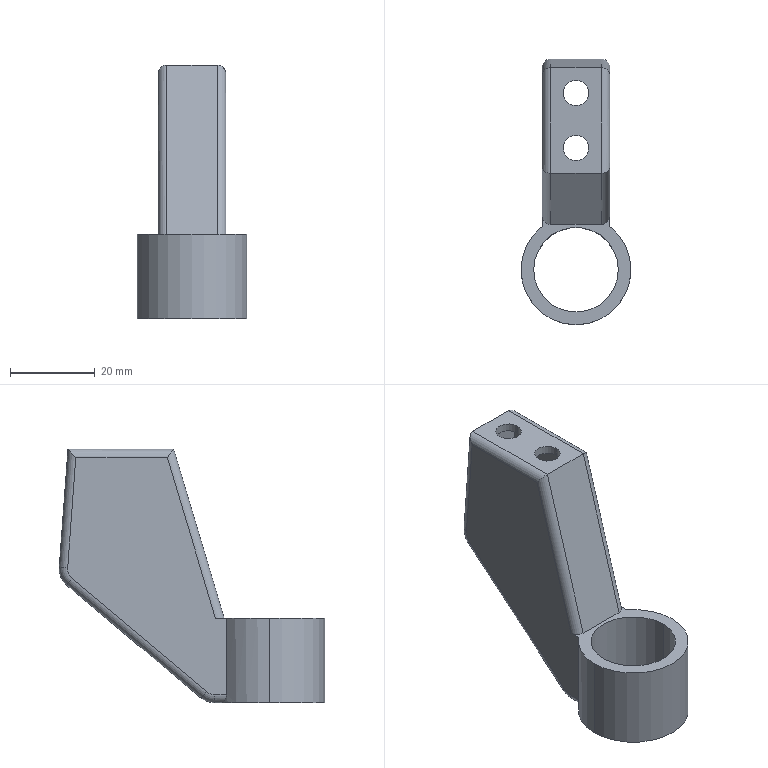Part | STEP file | Dual Brake Lever Body | 1 solid | 39 faces | box 26 x 62.825 x 60 mm | volume 18209 mm3 | cylinder 21 | plane 14 | torus 4 | commonest cylinder face diameters 4 x10 6 x4 26 x3 10 x2 20 x2